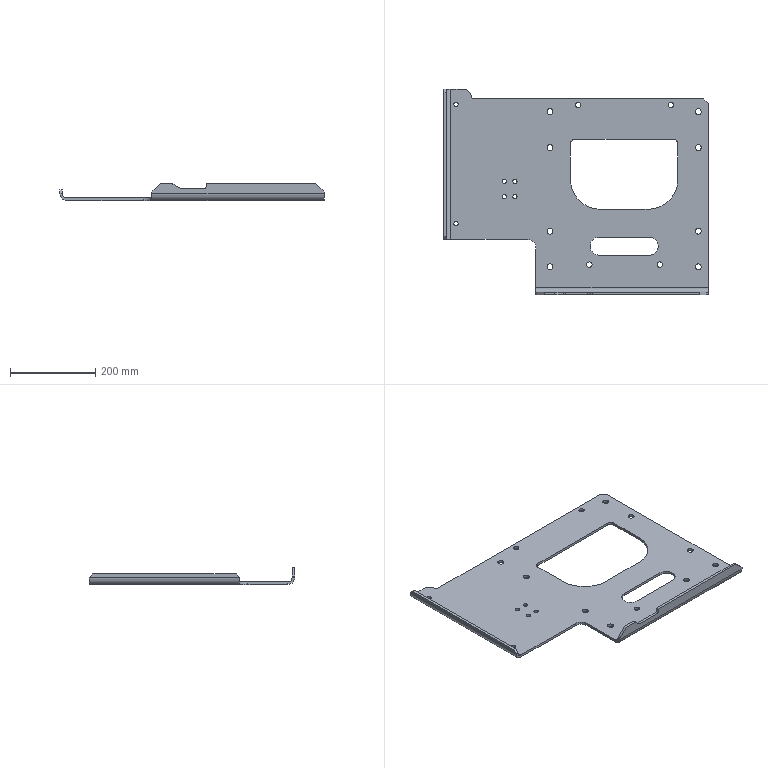Part | SolidWorks | features ICE 7, Chamfer 3, EdgeFlange 2, Fillet 2, SMBaseFlange 2, FlatPattern 1, SheetMetal 1 | 1 solid | 87 faces | box 620 x 481.4 x 40 mm | volume 1351039 mm3 | cylinder 53 | plane 34 | commonest cylinder face diameters 14 x16 10 x14 12.5 x8 20 x7 42.5 x3 32 x2